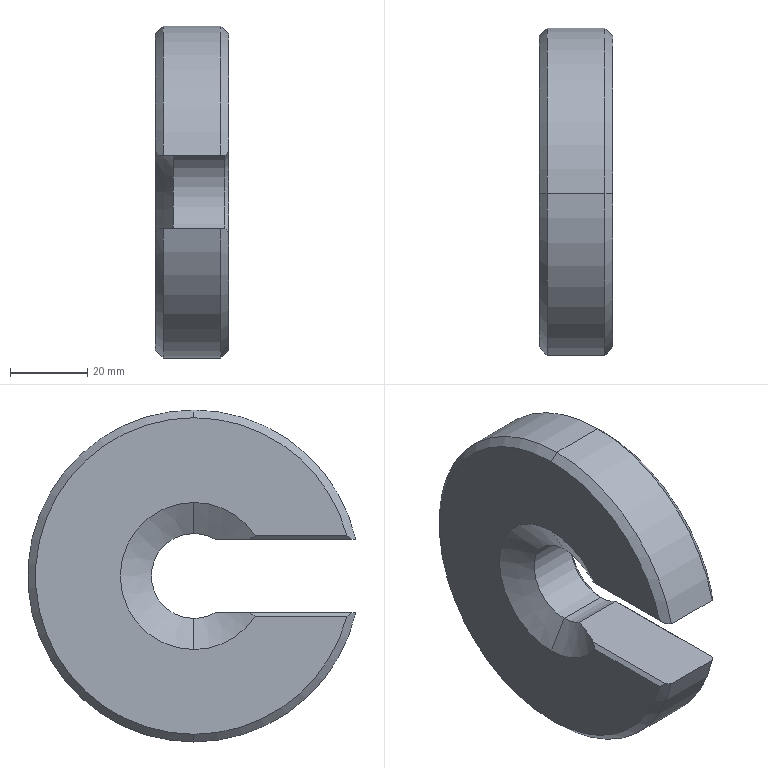Part | SolidWorks | features Chamfer 2, ICE 1, Revolution 1 | 1 solid | 26 faces | box 19 x 84.937 x 86 mm | volume 88865 mm3 | cone 12 | plane 8 | cylinder 6 | commonest cylinder face diameters 22 x3 86 x3
STEP:
#1=CARTESIAN_POINT('',(-1.,0.,11.));
#2=VERTEX_POINT('',#1);
#3=CARTESIAN_POINT('',(-1.,-5.545,9.5));
#4=VERTEX_POINT('',#3);
#5=CARTESIAN_POINT('',(-1.,0.,0.));
#6=DIRECTION('',(1.,0.,0.));
#7=DIRECTION('',(0.,0.,1.));
#8=AXIS2_PLACEMENT_3D('',#5,#6,#7);
#9=CIRCLE('',#8,11.);
#10=EDGE_CURVE('',#2,#4,#9,.T.);
#11=ORIENTED_EDGE('',*,*,#10,.F.);
#12=CARTESIAN_POINT('',(0.,0.,12.));
#13=VERTEX_POINT('',#12);
#14=CARTESIAN_POINT('',(0.,0.,12.));
#15=DIRECTION('',(0.7071,0.,0.7071));
#16=VECTOR('',#15,1000.);
#17=LINE('',#14,#16);
#18=EDGE_CURVE('',#2,#13,#17,.T.);
#19=ORIENTED_EDGE('',*,*,#18,.T.);
#20=CARTESIAN_POINT('',(0.,-5.809,10.5));
#21=VERTEX_POINT('',#20);
#22=CARTESIAN_POINT('',(0.,0.,0.));
#23=DIRECTION('',(-1.,0.,0.));
#24=DIRECTION('',(0.,0.,1.));
#25=AXIS2_PLACEMENT_3D('',#22,#23,#24);
#26=CIRCLE('',#25,12.);
#27=EDGE_CURVE('',#21,#13,#26,.T.);
#28=ORIENTED_EDGE('',*,*,#27,.F.);
#29=CARTESIAN_POINT('',(0.,-5.809,10.5));
#30=CARTESIAN_POINT('',(-0.3336,-5.723,10.166));
#31=CARTESIAN_POINT('',(-0.6669,-5.635,9.833));
#32=CARTESIAN_POINT('',(-1.,-5.545,9.5));
#33=B_SPLINE_CURVE_WITH_KNOTS('',3,(#29,#30,#31,#32),.UNSPECIFIED.,.F.,.F.,(4,4),(0.,0.001439),.UNSPECIFIED.);
#34=EDGE_CURVE('',#21,#4,#33,.T.);
#35=ORIENTED_EDGE('',*,*,#34,.T.);
#36=EDGE_LOOP('',(#11,#19,#28,#35));
#37=FACE_OUTER_BOUND('',#36,.T.);
#38=CARTESIAN_POINT('',(0.,0.,0.));
#39=DIRECTION('',(1.,0.,0.));
#40=DIRECTION('',(0.,0.,-1.));
#41=AXIS2_PLACEMENT_3D('',#38,#39,#40);
#42=CONICAL_SURFACE('',#41,12.,0.7854);
#43=ADVANCED_FACE('',(#37),#42,.F.);
#44=ORIENTED_EDGE('',*,*,#18,.F.);
#45=CARTESIAN_POINT('',(-1.,0.,-11.));
#46=VERTEX_POINT('',#45);
#47=CARTESIAN_POINT('',(-1.,0.,0.));
#48=DIRECTION('',(1.,0.,0.));
#49=DIRECTION('',(0.,0.,1.));
#50=AXIS2_PLACEMENT_3D('',#47,#48,#49);
#51=CIRCLE('',#50,11.);
#52=EDGE_CURVE('',#46,#2,#51,.T.);
#53=ORIENTED_EDGE('',*,*,#52,.F.);
#54=CARTESIAN_POINT('',(0.,0.,-12.));
#55=VERTEX_POINT('',#54);
#56=CARTESIAN_POINT('',(0.,0.,-12.));
#57=DIRECTION('',(0.7071,0.,-0.7071));
#58=VECTOR('',#57,1000.);
#59=LINE('',#56,#58);
#60=EDGE_CURVE('',#46,#55,#59,.T.);
#61=ORIENTED_EDGE('',*,*,#60,.T.);
#62=CARTESIAN_POINT('',(0.,0.,0.));
#63=DIRECTION('',(-1.,0.,0.));
#64=DIRECTION('',(0.,0.,1.));
#65=AXIS2_PLACEMENT_3D('',#62,#63,#64);
#66=CIRCLE('',#65,12.);
#67=EDGE_CURVE('',#13,#55,#66,.T.);
#68=ORIENTED_EDGE('',*,*,#67,.F.);
#69=EDGE_LOOP('',(#44,#53,#61,#68));
#70=FACE_OUTER_BOUND('',#69,.T.);
#71=CARTESIAN_POINT('',(0.,0.,0.));
#72=DIRECTION('',(1.,0.,0.));
#73=DIRECTION('',(0.,0.,-1.));
#74=AXIS2_PLACEMENT_3D('',#71,#72,#73);
#75=CONICAL_SURFACE('',#74,12.,0.7854);
#76=ADVANCED_FACE('',(#70),#75,.F.);
#77=CARTESIAN_POINT('',(-19.,0.,41.));
#78=VERTEX_POINT('',#77);
#79=CARTESIAN_POINT('',(-19.,0.,-41.));
#80=VERTEX_POINT('',#79);
#81=CARTESIAN_POINT('',(-19.,0.,0.));
#82=DIRECTION('',(-1.,0.,0.));
#83=DIRECTION('',(0.,0.,-1.));
#84=AXIS2_PLACEMENT_3D('',#81,#82,#83);
#85=CIRCLE('',#84,41.);
#86=EDGE_CURVE('',#78,#80,#85,.T.);
#87=ORIENTED_EDGE('',*,*,#86,.F.);
#88=CARTESIAN_POINT('',(-17.,0.,43.));
#89=VERTEX_POINT('',#88);
#90=CARTESIAN_POINT('',(-19.,0.,41.));
#91=DIRECTION('',(0.7071,0.,0.7071));
#92=VECTOR('',#91,1000.);
#93=LINE('',#90,#92);
#94=EDGE_CURVE('',#78,#89,#93,.T.);
#95=ORIENTED_EDGE('',*,*,#94,.T.);
#96=CARTESIAN_POINT('',(-17.,0.,-43.));
#97=VERTEX_POINT('',#96);
#98=CARTESIAN_POINT('',(-17.,0.,0.));
#99=DIRECTION('',(1.,0.,0.));
#100=DIRECTION('',(0.,0.,-1.));
#101=AXIS2_PLACEMENT_3D('',#98,#99,#100);
#102=CIRCLE('',#101,43.);
#103=EDGE_CURVE('',#97,#89,#102,.T.);
#104=ORIENTED_EDGE('',*,*,#103,.F.);
#105=CARTESIAN_POINT('',(-19.,0.,-41.));
#106=DIRECTION('',(0.7071,0.,-0.7071));
#107=VECTOR('',#106,1000.);
#108=LINE('',#105,#107);
#109=EDGE_CURVE('',#80,#97,#108,.T.);
#110=ORIENTED_EDGE('',*,*,#109,.F.);
#111=EDGE_LOOP('',(#87,#95,#104,#110));
#112=FACE_OUTER_BOUND('',#111,.T.);
#113=CARTESIAN_POINT('',(-19.,0.,0.));
#114=DIRECTION('',(1.,0.,0.));
#115=DIRECTION('',(0.,0.,-1.));
#116=AXIS2_PLACEMENT_3D('',#113,#114,#115);
#117=CONICAL_SURFACE('',#116,41.,0.7854);
#118=ADVANCED_FACE('',(#112),#117,.T.);
#119=CARTESIAN_POINT('',(-19.,-39.633,-10.5));
#120=VERTEX_POINT('',#119);
#121=CARTESIAN_POINT('',(-19.,0.,0.));
#122=DIRECTION('',(-1.,0.,0.));
#123=DIRECTION('',(0.,0.,-1.));
#124=AXIS2_PLACEMENT_3D('',#121,#122,#123);
#125=CIRCLE('',#124,41.);
#126=EDGE_CURVE('',#80,#120,#125,.T.);
#127=ORIENTED_EDGE('',*,*,#126,.F.);
#128=ORIENTED_EDGE('',*,*,#109,.T.);
#129=CARTESIAN_POINT('',(-17.,-41.937,-9.5));
#130=VERTEX_POINT('',#129);
#131=CARTESIAN_POINT('',(-17.,0.,0.));
#132=DIRECTION('',(1.,0.,0.));
#133=DIRECTION('',(0.,0.,-1.));
#134=AXIS2_PLACEMENT_3D('',#131,#132,#133);
#135=CIRCLE('',#134,43.);
#136=EDGE_CURVE('',#130,#97,#135,.T.);
#137=ORIENTED_EDGE('',*,*,#136,.F.);
#138=CARTESIAN_POINT('',(-18.,-40.911,-9.5));
#139=VERTEX_POINT('',#138);
#140=CARTESIAN_POINT('',(-18.,-40.911,-9.5));
#141=CARTESIAN_POINT('',(-17.667,-41.254,-9.5));
#142=CARTESIAN_POINT('',(-17.333,-41.596,-9.5));
#143=CARTESIAN_POINT('',(-17.,-41.937,-9.5));
#144=B_SPLINE_CURVE_WITH_KNOTS('',3,(#140,#141,#142,#143),.UNSPECIFIED.,.F.,.F.,(4,4),(0.03563,0.03706),.UNSPECIFIED.);
#145=EDGE_CURVE('',#139,#130,#144,.T.);
#146=ORIENTED_EDGE('',*,*,#145,.F.);
#147=CARTESIAN_POINT('',(-18.,-40.911,-9.5));
#148=CARTESIAN_POINT('',(-18.336,-40.489,-9.836));
#149=CARTESIAN_POINT('',(-18.669,-40.063,-10.169));
#150=CARTESIAN_POINT('',(-19.,-39.633,-10.5));
#151=B_SPLINE_CURVE_WITH_KNOTS('',3,(#147,#148,#149,#150),.UNSPECIFIED.,.F.,.F.,(4,4),(0.,0.001907),.UNSPECIFIED.);
#152=EDGE_CURVE('',#139,#120,#151,.T.);
#153=ORIENTED_EDGE('',*,*,#152,.T.);
#154=EDGE_LOOP('',(#127,#128,#137,#146,#153));
#155=FACE_OUTER_BOUND('',#154,.T.);
#156=CARTESIAN_POINT('',(-19.,0.,0.));
#157=DIRECTION('',(1.,0.,0.));
#158=DIRECTION('',(0.,0.,-1.));
#159=AXIS2_PLACEMENT_3D('',#156,#157,#158);
#160=CONICAL_SURFACE('',#159,41.,0.7854);
#161=ADVANCED_FACE('',(#155),#160,.T.);
#162=CARTESIAN_POINT('',(0.,0.,-41.));
#163=VERTEX_POINT('',#162);
#164=CARTESIAN_POINT('',(0.,0.,41.));
#165=VERTEX_POINT('',#164);
#166=CARTESIAN_POINT('',(0.,0.,0.));
#167=DIRECTION('',(1.,0.,0.));
#168=DIRECTION('',(0.,0.,1.));
#169=AXIS2_PLACEMENT_3D('',#166,#167,#168);
#170=CIRCLE('',#169,41.);
#171=EDGE_CURVE('',#163,#165,#170,.T.);
#172=ORIENTED_EDGE('',*,*,#171,.F.);
#173=CARTESIAN_POINT('',(-2.,0.,-43.));
#174=VERTEX_POINT('',#173);
#175=CARTESIAN_POINT('',(-2.,0.,-43.));
#176=DIRECTION('',(-0.7071,0.,-0.7071));
#177=VECTOR('',#176,1000.);
#178=LINE('',#175,#177);
#179=EDGE_CURVE('',#163,#174,#178,.T.);
#180=ORIENTED_EDGE('',*,*,#179,.T.);
#181=CARTESIAN_POINT('',(-2.,0.,43.));
#182=VERTEX_POINT('',#181);
#183=CARTESIAN_POINT('',(-2.,0.,0.));
#184=DIRECTION('',(-1.,0.,0.));
#185=DIRECTION('',(0.,0.,1.));
#186=AXIS2_PLACEMENT_3D('',#183,#184,#185);
#187=CIRCLE('',#186,43.);
#188=EDGE_CURVE('',#182,#174,#187,.T.);
#189=ORIENTED_EDGE('',*,*,#188,.F.);
#190=CARTESIAN_POINT('',(-2.,0.,43.));
#191=DIRECTION('',(-0.7071,0.,0.7071));
#192=VECTOR('',#191,1000.);
#193=LINE('',#190,#192);
#194=EDGE_CURVE('',#165,#182,#193,.T.);
#195=ORIENTED_EDGE('',*,*,#194,.F.);
#196=EDGE_LOOP('',(#172,#180,#189,#195));
#197=FACE_OUTER_BOUND('',#196,.T.);
#198=CARTESIAN_POINT('',(-2.,0.,0.));
#199=DIRECTION('',(-1.,0.,0.));
#200=DIRECTION('',(0.,0.,1.));
#201=AXIS2_PLACEMENT_3D('',#198,#199,#200);
#202=CONICAL_SURFACE('',#201,43.,0.7854);
#203=ADVANCED_FACE('',(#197),#202,.T.);
#204=CARTESIAN_POINT('',(0.,-39.633,10.5));
#205=VERTEX_POINT('',#204);
#206=CARTESIAN_POINT('',(0.,0.,0.));
#207=DIRECTION('',(1.,0.,0.));
#208=DIRECTION('',(0.,0.,1.));
#209=AXIS2_PLACEMENT_3D('',#206,#207,#208);
#210=CIRCLE('',#209,41.);
#211=EDGE_CURVE('',#165,#205,#210,.T.);
#212=ORIENTED_EDGE('',*,*,#211,.F.);
#213=ORIENTED_EDGE('',*,*,#194,.T.);
#214=CARTESIAN_POINT('',(-2.,-41.937,9.5));
#215=VERTEX_POINT('',#214);
#216=CARTESIAN_POINT('',(-2.,0.,0.));
#217=DIRECTION('',(-1.,0.,0.));
#218=DIRECTION('',(0.,0.,1.));
#219=AXIS2_PLACEMENT_3D('',#216,#217,#218);
#220=CIRCLE('',#219,43.);
#221=EDGE_CURVE('',#215,#182,#220,.T.);
#222=ORIENTED_EDGE('',*,*,#221,.F.);
#223=CARTESIAN_POINT('',(-1.,-40.911,9.5));
#224=VERTEX_POINT('',#223);
#225=CARTESIAN_POINT('',(-1.,-40.911,9.5));
#226=CARTESIAN_POINT('',(-1.333,-41.254,9.5));
#227=CARTESIAN_POINT('',(-1.667,-41.596,9.5));
#228=CARTESIAN_POINT('',(-2.,-41.937,9.5));
#229=B_SPLINE_CURVE_WITH_KNOTS('',3,(#225,#226,#227,#228),.UNSPECIFIED.,.F.,.F.,(4,4),(0.03563,0.03706),.UNSPECIFIED.);
#230=EDGE_CURVE('',#224,#215,#229,.T.);
#231=ORIENTED_EDGE('',*,*,#230,.F.);
#232=CARTESIAN_POINT('',(-1.,-40.911,9.5));
#233=CARTESIAN_POINT('',(-0.6643,-40.489,9.836));
#234=CARTESIAN_POINT('',(-0.3309,-40.063,10.169));
#235=CARTESIAN_POINT('',(0.,-39.633,10.5));
#236=B_SPLINE_CURVE_WITH_KNOTS('',3,(#232,#233,#234,#235),.UNSPECIFIED.,.F.,.F.,(4,4),(0.,0.001907),.UNSPECIFIED.);
#237=EDGE_CURVE('',#224,#205,#236,.T.);
#238=ORIENTED_EDGE('',*,*,#237,.T.);
#239=EDGE_LOOP('',(#212,#213,#222,#231,#238));
#240=FACE_OUTER_BOUND('',#239,.T.);
#241=CARTESIAN_POINT('',(-2.,0.,0.));
#242=DIRECTION('',(-1.,0.,0.));
#243=DIRECTION('',(0.,0.,1.));
#244=AXIS2_PLACEMENT_3D('',#241,#242,#243);
#245=CONICAL_SURFACE('',#244,43.,0.7854);
#246=ADVANCED_FACE('',(#240),#245,.T.);
#247=CARTESIAN_POINT('',(-14.35,0.,-11.));
#248=VERTEX_POINT('',#247);
#249=CARTESIAN_POINT('',(-14.35,-5.545,-9.5));
#250=VERTEX_POINT('',#249);
#251=CARTESIAN_POINT('',(-14.35,0.,0.));
#252=DIRECTION('',(-1.,0.,0.));
#253=DIRECTION('',(0.,0.,1.));
#254=AXIS2_PLACEMENT_3D('',#251,#252,#253);
#255=CIRCLE('',#254,11.);
#256=EDGE_CURVE('',#248,#250,#255,.T.);
#257=ORIENTED_EDGE('',*,*,#256,.F.);
#258=CARTESIAN_POINT('',(-19.,0.,-19.05));
#259=VERTEX_POINT('',#258);
#260=CARTESIAN_POINT('',(-19.,0.,-19.05));
#261=DIRECTION('',(-0.5002,0.,-0.8659));
#262=VECTOR('',#261,1000.);
#263=LINE('',#260,#262);
#264=EDGE_CURVE('',#248,#259,#263,.T.);
#265=ORIENTED_EDGE('',*,*,#264,.T.);
#266=CARTESIAN_POINT('',(-19.,-15.895,-10.5));
#267=VERTEX_POINT('',#266);
#268=CARTESIAN_POINT('',(-19.,0.,0.));
#269=DIRECTION('',(-1.,0.,0.));
#270=DIRECTION('',(0.,0.,1.));
#271=AXIS2_PLACEMENT_3D('',#268,#269,#270);
#272=CIRCLE('',#271,19.05);
#273=EDGE_CURVE('',#259,#267,#272,.T.);
#274=ORIENTED_EDGE('',*,*,#273,.T.);
#275=CARTESIAN_POINT('',(-18.,-14.481,-9.5));
#276=VERTEX_POINT('',#275);
#277=CARTESIAN_POINT('',(-19.,-15.895,-10.5));
#278=CARTESIAN_POINT('',(-18.667,-15.424,-10.167));
#279=CARTESIAN_POINT('',(-18.333,-14.952,-9.833));
#280=CARTESIAN_POINT('',(-18.,-14.481,-9.5));
#281=B_SPLINE_CURVE_WITH_KNOTS('',3,(#277,#278,#279,#280),.UNSPECIFIED.,.F.,.F.,(4,4),(0.,0.002),.UNSPECIFIED.);
#282=EDGE_CURVE('',#267,#276,#281,.T.);
#283=ORIENTED_EDGE('',*,*,#282,.T.);
#284=CARTESIAN_POINT('',(-18.,-14.481,-9.5));
#285=CARTESIAN_POINT('',(-17.299,-13.029,-9.5));
#286=CARTESIAN_POINT('',(-16.622,-11.567,-9.5));
#287=CARTESIAN_POINT('',(-15.687,-9.342,-9.5));
#288=CARTESIAN_POINT('',(-15.389,-8.595,-9.5));
#289=CARTESIAN_POINT('',(-14.833,-7.085,-9.5));
#290=CARTESIAN_POINT('',(-14.576,-6.321,-9.5));
#291=CARTESIAN_POINT('',(-14.35,-5.545,-9.5));
#292=B_SPLINE_CURVE_WITH_KNOTS('',3,(#284,#285,#286,#287,#288,#289,#290,#291),.UNSPECIFIED.,.F.,.F.,(4,2,2,4),(0.01847,0.0233,0.02572,0.02814),.UNSPECIFIED.);
#293=EDGE_CURVE('',#276,#250,#292,.T.);
#294=ORIENTED_EDGE('',*,*,#293,.T.);
#295=EDGE_LOOP('',(#257,#265,#274,#283,#294));
#296=FACE_OUTER_BOUND('',#295,.T.);
#297=CARTESIAN_POINT('',(-19.,0.,0.));
#298=DIRECTION('',(-1.,0.,0.));
#299=DIRECTION('',(0.,0.,1.));
#300=AXIS2_PLACEMENT_3D('',#297,#298,#299);
#301=CONICAL_SURFACE('',#300,19.05,1.047);
#302=ADVANCED_FACE('',(#296),#301,.F.);
#303=ORIENTED_EDGE('',*,*,#264,.F.);
#304=CARTESIAN_POINT('',(-14.35,0.,11.));
#305=VERTEX_POINT('',#304);
#306=CARTESIAN_POINT('',(-14.35,0.,0.));
#307=DIRECTION('',(-1.,0.,0.));
#308=DIRECTION('',(0.,0.,1.));
#309=AXIS2_PLACEMENT_3D('',#306,#307,#308);
#310=CIRCLE('',#309,11.);
#311=EDGE_CURVE('',#305,#248,#310,.T.);
#312=ORIENTED_EDGE('',*,*,#311,.F.);
#313=CARTESIAN_POINT('',(-19.,0.,19.05));
#314=VERTEX_POINT('',#313);
#315=CARTESIAN_POINT('',(-19.,0.,19.05));
#316=DIRECTION('',(-0.5002,0.,0.8659));
#317=VECTOR('',#316,1000.);
#318=LINE('',#315,#317);
#319=EDGE_CURVE('',#305,#314,#318,.T.);
#320=ORIENTED_EDGE('',*,*,#319,.T.);
#321=CARTESIAN_POINT('',(-19.,0.,0.));
#322=DIRECTION('',(-1.,0.,0.));
#323=DIRECTION('',(0.,0.,1.));
#324=AXIS2_PLACEMENT_3D('',#321,#322,#323);
#325=CIRCLE('',#324,19.05);
#326=EDGE_CURVE('',#314,#259,#325,.T.);
#327=ORIENTED_EDGE('',*,*,#326,.T.);
#328=EDGE_LOOP('',(#303,#312,#320,#327));
#329=FACE_OUTER_BOUND('',#328,.T.);
#330=CARTESIAN_POINT('',(-19.,0.,0.));
#331=DIRECTION('',(-1.,0.,0.));
#332=DIRECTION('',(0.,0.,1.));
#333=AXIS2_PLACEMENT_3D('',#330,#331,#332);
#334=CONICAL_SURFACE('',#333,19.05,1.047);
#335=ADVANCED_FACE('',(#329),#334,.F.);
#336=CARTESIAN_POINT('',(-1.,-5.545,-9.5));
#337=VERTEX_POINT('',#336);
#338=CARTESIAN_POINT('',(-1.,0.,0.));
#339=DIRECTION('',(1.,0.,0.));
#340=DIRECTION('',(0.,0.,1.));
#341=AXIS2_PLACEMENT_3D('',#338,#339,#340);
#342=CIRCLE('',#341,11.);
#343=EDGE_CURVE('',#337,#46,#342,.T.);
#344=ORIENTED_EDGE('',*,*,#343,.T.);
#345=CARTESIAN_POINT('',(-44.951,0.,-11.));
#346=DIRECTION('',(-1.,0.,0.));
#347=VECTOR('',#346,1000.);
#348=LINE('',#345,#347);
#349=EDGE_CURVE('',#46,#248,#348,.T.);
#350=ORIENTED_EDGE('',*,*,#349,.T.);
#351=ORIENTED_EDGE('',*,*,#256,.T.);
#352=CARTESIAN_POINT('',(-44.951,-5.545,-9.5));
#353=DIRECTION('',(1.,0.,0.));
#354=VECTOR('',#353,1000.);
#355=LINE('',#352,#354);
#356=EDGE_CURVE('',#250,#337,#355,.T.);
#357=ORIENTED_EDGE('',*,*,#356,.T.);
#358=EDGE_LOOP('',(#344,#350,#351,#357));
#359=FACE_OUTER_BOUND('',#358,.T.);
#360=CARTESIAN_POINT('',(-44.951,0.,0.));
#361=DIRECTION('',(-1.,0.,0.));
#362=DIRECTION('',(0.,0.,1.));
#363=AXIS2_PLACEMENT_3D('',#360,#361,#362);
#364=CYLINDRICAL_SURFACE('',#363,11.);
#365=ADVANCED_FACE('',(#359),#364,.F.);
#366=ORIENTED_EDGE('',*,*,#349,.F.);
#367=ORIENTED_EDGE('',*,*,#52,.T.);
#368=CARTESIAN_POINT('',(-44.951,0.,11.));
#369=DIRECTION('',(-1.,0.,0.));
#370=VECTOR('',#369,1000.);
#371=LINE('',#368,#370);
#372=EDGE_CURVE('',#2,#305,#371,.T.);
#373=ORIENTED_EDGE('',*,*,#372,.T.);
#374=ORIENTED_EDGE('',*,*,#311,.T.);
#375=EDGE_LOOP('',(#366,#367,#373,#374));
#376=FACE_OUTER_BOUND('',#375,.T.);
#377=CARTESIAN_POINT('',(-44.951,0.,0.));
#378=DIRECTION('',(-1.,0.,0.));
#379=DIRECTION('',(0.,0.,1.));
#380=AXIS2_PLACEMENT_3D('',#377,#378,#379);
#381=CYLINDRICAL_SURFACE('',#380,11.);
#382=ADVANCED_FACE('',(#376),#381,.F.);
#383=ORIENTED_EDGE('',*,*,#188,.T.);
#384=CARTESIAN_POINT('',(-44.951,0.,-43.));
#385=DIRECTION('',(-1.,0.,0.));
#386=VECTOR('',#385,1000.);
#387=LINE('',#384,#386);
#388=EDGE_CURVE('',#174,#97,#387,.T.);
#389=ORIENTED_EDGE('',*,*,#388,.T.);
#390=ORIENTED_EDGE('',*,*,#103,.T.);
#391=CARTESIAN_POINT('',(-44.951,0.,43.));
#392=DIRECTION('',(-1.,0.,0.));
#393=VECTOR('',#392,1000.);
#394=LINE('',#391,#393);
#395=EDGE_CURVE('',#182,#89,#394,.T.);
#396=ORIENTED_EDGE('',*,*,#395,.F.);
#397=EDGE_LOOP('',(#383,#389,#390,#396));
#398=FACE_OUTER_BOUND('',#397,.T.);
#399=CARTESIAN_POINT('',(-44.951,0.,0.));
#400=DIRECTION('',(-1.,0.,0.));
#401=DIRECTION('',(0.,0.,1.));
#402=AXIS2_PLACEMENT_3D('',#399,#400,#401);
#403=CYLINDRICAL_SURFACE('',#402,43.);
#404=ADVANCED_FACE('',(#398),#403,.T.);
#405=ORIENTED_EDGE('',*,*,#221,.T.);
#406=ORIENTED_EDGE('',*,*,#395,.T.);
#407=CARTESIAN_POINT('',(-17.,-41.937,9.5));
#408=VERTEX_POINT('',#407);
#409=CARTESIAN_POINT('',(-17.,0.,0.));
#410=DIRECTION('',(1.,0.,0.));
#411=DIRECTION('',(0.,0.,-1.));
#412=AXIS2_PLACEMENT_3D('',#409,#410,#411);
#413=CIRCLE('',#412,43.);
#414=EDGE_CURVE('',#89,#408,#413,.T.);
#415=ORIENTED_EDGE('',*,*,#414,.T.);
#416=CARTESIAN_POINT('',(-44.951,-41.937,9.5));
#417=DIRECTION('',(1.,0.,0.));
#418=VECTOR('',#417,1000.);
#419=LINE('',#416,#418);
#420=EDGE_CURVE('',#408,#215,#419,.T.);
#421=ORIENTED_EDGE('',*,*,#420,.T.);
#422=EDGE_LOOP('',(#405,#406,#415,#421));
#423=FACE_OUTER_BOUND('',#422,.T.);
#424=CARTESIAN_POINT('',(-44.951,0.,0.));
#425=DIRECTION('',(-1.,0.,0.));
#426=DIRECTION('',(0.,0.,1.));
#427=AXIS2_PLACEMENT_3D('',#424,#425,#426);
#428=CYLINDRICAL_SURFACE('',#427,43.);
#429=ADVANCED_FACE('',(#423),#428,.T.);
#430=ORIENTED_EDGE('',*,*,#388,.F.);
#431=CARTESIAN_POINT('',(-2.,-41.937,-9.5));
#432=VERTEX_POINT('',#431);
#433=CARTESIAN_POINT('',(-2.,0.,0.));
#434=DIRECTION('',(-1.,0.,0.));
#435=DIRECTION('',(0.,0.,1.));
#436=AXIS2_PLACEMENT_3D('',#433,#434,#435);
#437=CIRCLE('',#436,43.);
#438=EDGE_CURVE('',#174,#432,#437,.T.);
#439=ORIENTED_EDGE('',*,*,#438,.T.);
#440=CARTESIAN_POINT('',(-44.951,-41.937,-9.5));
#441=DIRECTION('',(-1.,0.,0.));
#442=VECTOR('',#441,1000.);
#443=LINE('',#440,#442);
#444=EDGE_CURVE('',#432,#130,#443,.T.);
#445=ORIENTED_EDGE('',*,*,#444,.T.);
#446=ORIENTED_EDGE('',*,*,#136,.T.);
#447=EDGE_LOOP('',(#430,#439,#445,#446));
#448=FACE_OUTER_BOUND('',#447,.T.);
#449=CARTESIAN_POINT('',(-44.951,0.,0.));
#450=DIRECTION('',(-1.,0.,0.));
#451=DIRECTION('',(0.,0.,1.));
#452=AXIS2_PLACEMENT_3D('',#449,#450,#451);
#453=CYLINDRICAL_SURFACE('',#452,43.);
#454=ADVANCED_FACE('',(#448),#453,.T.);
#455=ORIENTED_EDGE('',*,*,#27,.T.);
#456=ORIENTED_EDGE('',*,*,#67,.T.);
#457=CARTESIAN_POINT('',(0.,-5.809,-10.5));
#458=VERTEX_POINT('',#457);
#459=CARTESIAN_POINT('',(0.,0.,0.));
#460=DIRECTION('',(-1.,0.,0.));
#461=DIRECTION('',(0.,0.,1.));
#462=AXIS2_PLACEMENT_3D('',#459,#460,#461);
#463=CIRCLE('',#462,12.);
#464=EDGE_CURVE('',#55,#458,#463,.T.);
#465=ORIENTED_EDGE('',*,*,#464,.T.);
#466=CARTESIAN_POINT('',(0.,-39.633,-10.5));
#467=VERTEX_POINT('',#466);
#468=CARTESIAN_POINT('',(0.,43.,-10.5));
#469=DIRECTION('',(0.,-1.,0.));
#470=VECTOR('',#469,1000.);
#471=LINE('',#468,#470);
#472=EDGE_CURVE('',#458,#467,#471,.T.);
#473=ORIENTED_EDGE('',*,*,#472,.T.);
#474=CARTESIAN_POINT('',(0.,0.,0.));
#475=DIRECTION('',(1.,0.,0.));
#476=DIRECTION('',(0.,0.,1.));
#477=AXIS2_PLACEMENT_3D('',#474,#475,#476);
#478=CIRCLE('',#477,41.);
#479=EDGE_CURVE('',#467,#163,#478,.T.);
#480=ORIENTED_EDGE('',*,*,#479,.T.);
#481=ORIENTED_EDGE('',*,*,#171,.T.);
#482=ORIENTED_EDGE('',*,*,#211,.T.);
#483=CARTESIAN_POINT('',(0.,43.,10.5));
#484=DIRECTION('',(0.,1.,0.));
#485=VECTOR('',#484,1000.);
#486=LINE('',#483,#485);
#487=EDGE_CURVE('',#205,#21,#486,.T.);
#488=ORIENTED_EDGE('',*,*,#487,.T.);
#489=EDGE_LOOP('',(#455,#456,#465,#473,#480,#481,#482,#488));
#490=FACE_OUTER_BOUND('',#489,.T.);
#491=CARTESIAN_POINT('',(0.,43.,0.));
#492=DIRECTION('',(-1.,0.,0.));
#493=DIRECTION('',(0.,0.,1.));
#494=AXIS2_PLACEMENT_3D('',#491,#492,#493);
#495=PLANE('',#494);
#496=ADVANCED_FACE('',(#490),#495,.F.);
#497=ORIENTED_EDGE('',*,*,#372,.F.);
#498=ORIENTED_EDGE('',*,*,#10,.T.);
#499=CARTESIAN_POINT('',(-14.35,-5.545,9.5));
#500=VERTEX_POINT('',#499);
#501=CARTESIAN_POINT('',(-44.951,-5.545,9.5));
#502=DIRECTION('',(-1.,0.,0.));
#503=VECTOR('',#502,1000.);
#504=LINE('',#501,#503);
#505=EDGE_CURVE('',#4,#500,#504,.T.);
#506=ORIENTED_EDGE('',*,*,#505,.T.);
#507=CARTESIAN_POINT('',(-14.35,0.,0.));
#508=DIRECTION('',(-1.,0.,0.));
#509=DIRECTION('',(0.,0.,1.));
#510=AXIS2_PLACEMENT_3D('',#507,#508,#509);
#511=CIRCLE('',#510,11.);
#512=EDGE_CURVE('',#500,#305,#511,.T.);
#513=ORIENTED_EDGE('',*,*,#512,.T.);
#514=EDGE_LOOP('',(#497,#498,#506,#513));
#515=FACE_OUTER_BOUND('',#514,.T.);
#516=CARTESIAN_POINT('',(-44.951,0.,0.));
#517=DIRECTION('',(-1.,0.,0.));
#518=DIRECTION('',(0.,0.,1.));
#519=AXIS2_PLACEMENT_3D('',#516,#517,#518);
#520=CYLINDRICAL_SURFACE('',#519,11.);
#521=ADVANCED_FACE('',(#515),#520,.F.);
#522=ORIENTED_EDGE('',*,*,#319,.F.);
#523=ORIENTED_EDGE('',*,*,#512,.F.);
#524=CARTESIAN_POINT('',(-18.,-14.481,9.5));
#525=VERTEX_POINT('',#524);
#526=CARTESIAN_POINT('',(-14.35,-5.545,9.5));
#527=CARTESIAN_POINT('',(-14.576,-6.32,9.5));
#528=CARTESIAN_POINT('',(-14.833,-7.083,9.5));
#529=CARTESIAN_POINT('',(-15.388,-8.593,9.5));
#530=CARTESIAN_POINT('',(-15.686,-9.34,9.5));
#531=CARTESIAN_POINT('',(-16.621,-11.565,9.5));
#532=CARTESIAN_POINT('',(-17.298,-13.028,9.5));
#533=CARTESIAN_POINT('',(-18.,-14.481,9.5));
#534=B_SPLINE_CURVE_WITH_KNOTS('',3,(#526,#527,#528,#529,#530,#531,#532,#533),.UNSPECIFIED.,.F.,.F.,(4,2,2,4),(0.01791,0.02034,0.02277,0.02763),.UNSPECIFIED.);
#535=EDGE_CURVE('',#500,#525,#534,.T.);
#536=ORIENTED_EDGE('',*,*,#535,.T.);
#537=CARTESIAN_POINT('',(-19.,-15.895,10.5));
#538=VERTEX_POINT('',#537);
#539=CARTESIAN_POINT('',(-18.,-14.481,9.5));
#540=CARTESIAN_POINT('',(-18.333,-14.952,9.833));
#541=CARTESIAN_POINT('',(-18.667,-15.424,10.167));
#542=CARTESIAN_POINT('',(-19.,-15.895,10.5));
#543=B_SPLINE_CURVE_WITH_KNOTS('',3,(#539,#540,#541,#542),.UNSPECIFIED.,.F.,.F.,(4,4),(0.,0.002),.UNSPECIFIED.);
#544=EDGE_CURVE('',#525,#538,#543,.T.);
#545=ORIENTED_EDGE('',*,*,#544,.T.);
#546=CARTESIAN_POINT('',(-19.,0.,0.));
#547=DIRECTION('',(-1.,0.,0.));
#548=DIRECTION('',(0.,0.,1.));
#549=AXIS2_PLACEMENT_3D('',#546,#547,#548);
#550=CIRCLE('',#549,19.05);
#551=EDGE_CURVE('',#538,#314,#550,.T.);
#552=ORIENTED_EDGE('',*,*,#551,.T.);
#553=EDGE_LOOP('',(#522,#523,#536,#545,#552));
#554=FACE_OUTER_BOUND('',#553,.T.);
#555=CARTESIAN_POINT('',(-19.,0.,0.));
#556=DIRECTION('',(-1.,0.,0.));
#557=DIRECTION('',(0.,0.,1.));
#558=AXIS2_PLACEMENT_3D('',#555,#556,#557);
#559=CONICAL_SURFACE('',#558,19.05,1.047);
#560=ADVANCED_FACE('',(#554),#559,.F.);
#561=CARTESIAN_POINT('',(-19.,-39.633,10.5));
#562=VERTEX_POINT('',#561);
#563=CARTESIAN_POINT('',(-19.,0.,0.));
#564=DIRECTION('',(-1.,0.,0.));
#565=DIRECTION('',(0.,0.,-1.));
#566=AXIS2_PLACEMENT_3D('',#563,#564,#565);
#567=CIRCLE('',#566,41.);
#568=EDGE_CURVE('',#562,#78,#567,.T.);
#569=ORIENTED_EDGE('',*,*,#568,.T.);
#570=ORIENTED_EDGE('',*,*,#86,.T.);
#571=ORIENTED_EDGE('',*,*,#126,.T.);
#572=CARTESIAN_POINT('',(-19.,19.05,-10.5));
#573=DIRECTION('',(0.,1.,0.));
#574=VECTOR('',#573,1000.);
#575=LINE('',#572,#574);
#576=EDGE_CURVE('',#120,#267,#575,.T.);
#577=ORIENTED_EDGE('',*,*,#576,.T.);
#578=ORIENTED_EDGE('',*,*,#273,.F.);
#579=ORIENTED_EDGE('',*,*,#326,.F.);
#580=ORIENTED_EDGE('',*,*,#551,.F.);
#581=CARTESIAN_POINT('',(-19.,19.05,10.5));
#582=DIRECTION('',(0.,-1.,0.));
#583=VECTOR('',#582,1000.);
#584=LINE('',#581,#583);
#585=EDGE_CURVE('',#538,#562,#584,.T.);
#586=ORIENTED_EDGE('',*,*,#585,.T.);
#587=EDGE_LOOP('',(#569,#570,#571,#577,#578,#579,#580,#586));
#588=FACE_OUTER_BOUND('',#587,.T.);
#589=CARTESIAN_POINT('',(-19.,19.05,0.));
#590=DIRECTION('',(1.,0.,0.));
#591=DIRECTION('',(0.,0.,-1.));
#592=AXIS2_PLACEMENT_3D('',#589,#590,#591);
#593=PLANE('',#592);
#594=ADVANCED_FACE('',(#588),#593,.F.);
#595=ORIENTED_EDGE('',*,*,#179,.F.);
#596=ORIENTED_EDGE('',*,*,#479,.F.);
#597=CARTESIAN_POINT('',(-1.,-40.911,-9.5));
#598=VERTEX_POINT('',#597);
#599=CARTESIAN_POINT('',(0.,-39.633,-10.5));
#600=CARTESIAN_POINT('',(-0.3309,-40.063,-10.169));
#601=CARTESIAN_POINT('',(-0.6643,-40.489,-9.836));
#602=CARTESIAN_POINT('',(-1.,-40.911,-9.5));
#603=B_SPLINE_CURVE_WITH_KNOTS('',3,(#599,#600,#601,#602),.UNSPECIFIED.,.F.,.F.,(4,4),(0.,0.001907),.UNSPECIFIED.);
#604=EDGE_CURVE('',#467,#598,#603,.T.);
#605=ORIENTED_EDGE('',*,*,#604,.T.);
#606=CARTESIAN_POINT('',(-2.,-41.937,-9.5));
#607=CARTESIAN_POINT('',(-1.667,-41.596,-9.5));
#608=CARTESIAN_POINT('',(-1.333,-41.254,-9.5));
#609=CARTESIAN_POINT('',(-1.,-40.911,-9.5));
#610=B_SPLINE_CURVE_WITH_KNOTS('',3,(#606,#607,#608,#609),.UNSPECIFIED.,.F.,.F.,(4,4),(0.04349,0.04492),.UNSPECIFIED.);
#611=EDGE_CURVE('',#432,#598,#610,.T.);
#612=ORIENTED_EDGE('',*,*,#611,.F.);
#613=ORIENTED_EDGE('',*,*,#438,.F.);
#614=EDGE_LOOP('',(#595,#596,#605,#612,#613));
#615=FACE_OUTER_BOUND('',#614,.T.);
#616=CARTESIAN_POINT('',(-2.,0.,0.));
#617=DIRECTION('',(-1.,0.,0.));
#618=DIRECTION('',(0.,0.,1.));
#619=AXIS2_PLACEMENT_3D('',#616,#617,#618);
#620=CONICAL_SURFACE('',#619,43.,0.7854);
#621=ADVANCED_FACE('',(#615),#620,.T.);
#622=ORIENTED_EDGE('',*,*,#94,.F.);
#623=ORIENTED_EDGE('',*,*,#568,.F.);
#624=CARTESIAN_POINT('',(-18.,-40.911,9.5));
#625=VERTEX_POINT('',#624);
#626=CARTESIAN_POINT('',(-19.,-39.633,10.5));
#627=CARTESIAN_POINT('',(-18.669,-40.063,10.169));
#628=CARTESIAN_POINT('',(-18.336,-40.489,9.836));
#629=CARTESIAN_POINT('',(-18.,-40.911,9.5));
#630=B_SPLINE_CURVE_WITH_KNOTS('',3,(#626,#627,#628,#629),.UNSPECIFIED.,.F.,.F.,(4,4),(0.,0.001907),.UNSPECIFIED.);
#631=EDGE_CURVE('',#562,#625,#630,.T.);
#632=ORIENTED_EDGE('',*,*,#631,.T.);
#633=CARTESIAN_POINT('',(-17.,-41.937,9.5));
#634=CARTESIAN_POINT('',(-17.333,-41.596,9.5));
#635=CARTESIAN_POINT('',(-17.667,-41.254,9.5));
#636=CARTESIAN_POINT('',(-18.,-40.911,9.5));
#637=B_SPLINE_CURVE_WITH_KNOTS('',3,(#633,#634,#635,#636),.UNSPECIFIED.,.F.,.F.,(4,4),(0.04349,0.04492),.UNSPECIFIED.);
#638=EDGE_CURVE('',#408,#625,#637,.T.);
#639=ORIENTED_EDGE('',*,*,#638,.F.);
#640=ORIENTED_EDGE('',*,*,#414,.F.);
#641=EDGE_LOOP('',(#622,#623,#632,#639,#640));
#642=FACE_OUTER_BOUND('',#641,.T.);
#643=CARTESIAN_POINT('',(-19.,0.,0.));
#644=DIRECTION('',(1.,0.,0.));
#645=DIRECTION('',(0.,0.,-1.));
#646=AXIS2_PLACEMENT_3D('',#643,#644,#645);
#647=CONICAL_SURFACE('',#646,41.,0.7854);
#648=ADVANCED_FACE('',(#642),#647,.T.);
#649=ORIENTED_EDGE('',*,*,#293,.F.);
#650=CARTESIAN_POINT('',(-18.,0.,-9.5));
#651=DIRECTION('',(0.,-1.,0.));
#652=VECTOR('',#651,1000.);
#653=LINE('',#650,#652);
#654=EDGE_CURVE('',#276,#139,#653,.T.);
#655=ORIENTED_EDGE('',*,*,#654,.T.);
#656=ORIENTED_EDGE('',*,*,#145,.T.);
#657=ORIENTED_EDGE('',*,*,#444,.F.);
#658=ORIENTED_EDGE('',*,*,#611,.T.);
#659=CARTESIAN_POINT('',(-1.,0.,-9.5));
#660=DIRECTION('',(0.,1.,0.));
#661=VECTOR('',#660,1000.);
#662=LINE('',#659,#661);
#663=EDGE_CURVE('',#598,#337,#662,.T.);
#664=ORIENTED_EDGE('',*,*,#663,.T.);
#665=ORIENTED_EDGE('',*,*,#356,.F.);
#666=EDGE_LOOP('',(#649,#655,#656,#657,#658,#664,#665));
#667=FACE_OUTER_BOUND('',#666,.T.);
#668=CARTESIAN_POINT('',(24.,0.,-9.5));
#669=DIRECTION('',(0.,0.,-1.));
#670=DIRECTION('',(0.,1.,0.));
#671=AXIS2_PLACEMENT_3D('',#668,#669,#670);
#672=PLANE('',#671);
#673=ADVANCED_FACE('',(#667),#672,.F.);
#674=ORIENTED_EDGE('',*,*,#638,.T.);
#675=CARTESIAN_POINT('',(-18.,0.,9.5));
#676=DIRECTION('',(0.,1.,0.));
#677=VECTOR('',#676,1000.);
#678=LINE('',#675,#677);
#679=EDGE_CURVE('',#625,#525,#678,.T.);
#680=ORIENTED_EDGE('',*,*,#679,.T.);
#681=ORIENTED_EDGE('',*,*,#535,.F.);
#682=ORIENTED_EDGE('',*,*,#505,.F.);
#683=CARTESIAN_POINT('',(-1.,0.,9.5));
#684=DIRECTION('',(0.,-1.,0.));
#685=VECTOR('',#684,1000.);
#686=LINE('',#683,#685);
#687=EDGE_CURVE('',#4,#224,#686,.T.);
#688=ORIENTED_EDGE('',*,*,#687,.T.);
#689=ORIENTED_EDGE('',*,*,#230,.T.);
#690=ORIENTED_EDGE('',*,*,#420,.F.);
#691=EDGE_LOOP('',(#674,#680,#681,#682,#688,#689,#690));
#692=FACE_OUTER_BOUND('',#691,.T.);
#693=CARTESIAN_POINT('',(24.,0.,9.5));
#694=DIRECTION('',(0.,0.,1.));
#695=DIRECTION('',(0.,-1.,0.));
#696=AXIS2_PLACEMENT_3D('',#693,#694,#695);
#697=PLANE('',#696);
#698=ADVANCED_FACE('',(#692),#697,.F.);
#699=ORIENTED_EDGE('',*,*,#282,.F.);
#700=ORIENTED_EDGE('',*,*,#576,.F.);
#701=ORIENTED_EDGE('',*,*,#152,.F.);
#702=ORIENTED_EDGE('',*,*,#654,.F.);
#703=EDGE_LOOP('',(#699,#700,#701,#702));
#704=FACE_OUTER_BOUND('',#703,.T.);
#705=CARTESIAN_POINT('',(-18.,0.,-9.5));
#706=DIRECTION('',(0.7071,0.,-0.7071));
#707=DIRECTION('',(0.,-1.,0.));
#708=AXIS2_PLACEMENT_3D('',#705,#706,#707);
#709=PLANE('',#708);
#710=ADVANCED_FACE('',(#704),#709,.F.);
#711=ORIENTED_EDGE('',*,*,#631,.F.);
#712=ORIENTED_EDGE('',*,*,#585,.F.);
#713=ORIENTED_EDGE('',*,*,#544,.F.);
#714=ORIENTED_EDGE('',*,*,#679,.F.);
#715=EDGE_LOOP('',(#711,#712,#713,#714));
#716=FACE_OUTER_BOUND('',#715,.T.);
#717=CARTESIAN_POINT('',(-18.,0.,9.5));
#718=DIRECTION('',(0.7071,0.,0.7071));
#719=DIRECTION('',(0.,1.,0.));
#720=AXIS2_PLACEMENT_3D('',#717,#718,#719);
#721=PLANE('',#720);
#722=ADVANCED_FACE('',(#716),#721,.F.);
#723=ORIENTED_EDGE('',*,*,#237,.F.);
#724=ORIENTED_EDGE('',*,*,#687,.F.);
#725=ORIENTED_EDGE('',*,*,#34,.F.);
#726=ORIENTED_EDGE('',*,*,#487,.F.);
#727=EDGE_LOOP('',(#723,#724,#725,#726));
#728=FACE_OUTER_BOUND('',#727,.T.);
#729=CARTESIAN_POINT('',(0.,43.,10.5));
#730=DIRECTION('',(-0.7071,0.,0.7071));
#731=DIRECTION('',(0.,1.,0.));
#732=AXIS2_PLACEMENT_3D('',#729,#730,#731);
#733=PLANE('',#732);
#734=ADVANCED_FACE('',(#728),#733,.F.);
#735=ORIENTED_EDGE('',*,*,#60,.F.);
#736=ORIENTED_EDGE('',*,*,#343,.F.);
#737=CARTESIAN_POINT('',(0.,-5.809,-10.5));
#738=CARTESIAN_POINT('',(-0.3336,-5.723,-10.166));
#739=CARTESIAN_POINT('',(-0.6669,-5.635,-9.833));
#740=CARTESIAN_POINT('',(-1.,-5.545,-9.5));
#741=B_SPLINE_CURVE_WITH_KNOTS('',3,(#737,#738,#739,#740),.UNSPECIFIED.,.F.,.F.,(4,4),(0.,0.001439),.UNSPECIFIED.);
#742=EDGE_CURVE('',#458,#337,#741,.T.);
#743=ORIENTED_EDGE('',*,*,#742,.F.);
#744=ORIENTED_EDGE('',*,*,#464,.F.);
#745=EDGE_LOOP('',(#735,#736,#743,#744));
#746=FACE_OUTER_BOUND('',#745,.T.);
#747=CARTESIAN_POINT('',(0.,0.,0.));
#748=DIRECTION('',(1.,0.,0.));
#749=DIRECTION('',(0.,0.,-1.));
#750=AXIS2_PLACEMENT_3D('',#747,#748,#749);
#751=CONICAL_SURFACE('',#750,12.,0.7854);
#752=ADVANCED_FACE('',(#746),#751,.F.);
#753=ORIENTED_EDGE('',*,*,#742,.T.);
#754=ORIENTED_EDGE('',*,*,#663,.F.);
#755=ORIENTED_EDGE('',*,*,#604,.F.);
#756=ORIENTED_EDGE('',*,*,#472,.F.);
#757=EDGE_LOOP('',(#753,#754,#755,#756));
#758=FACE_OUTER_BOUND('',#757,.T.);
#759=CARTESIAN_POINT('',(0.,43.,-10.5));
#760=DIRECTION('',(-0.7071,0.,-0.7071));
#761=DIRECTION('',(0.,-1.,0.));
#762=AXIS2_PLACEMENT_3D('',#759,#760,#761);
#763=PLANE('',#762);
#764=ADVANCED_FACE('',(#758),#763,.F.);
#765=CLOSED_SHELL('',(#43,#76,#118,#161,#203,#246,#302,#335,#365,#382,#404,#429,#454,#496,#521,#560,#594,#621,#648,#673,#698,#710,#722,#734,#752,#764));
#766=MANIFOLD_SOLID_BREP('',#765);
#767=CARTESIAN_POINT('',(0.,0.,0.));
#768=DIRECTION('',(0.,0.,1.));
#769=DIRECTION('',(1.,0.,0.));
#770=AXIS2_PLACEMENT_3D('',#767,#768,#769);
#771=(LENGTH_UNIT()NAMED_UNIT(*)SI_UNIT(.MILLI.,.METRE.));
#772=UNCERTAINTY_MEASURE_WITH_UNIT(LENGTH_MEASURE(0.00001),#771,'','');
#773=(NAMED_UNIT(*)PLANE_ANGLE_UNIT()SI_UNIT($,.RADIAN.));
#774=(NAMED_UNIT(*)SI_UNIT($,.STERADIAN.)SOLID_ANGLE_UNIT());
#775=(GEOMETRIC_REPRESENTATION_CONTEXT(3)GLOBAL_UNCERTAINTY_ASSIGNED_CONTEXT((#772))GLOBAL_UNIT_ASSIGNED_CONTEXT((#771,#773,#774))REPRESENTATION_CONTEXT('',''));
#776=ADVANCED_BREP_SHAPE_REPRESENTATION('',(#766,#770),#775);